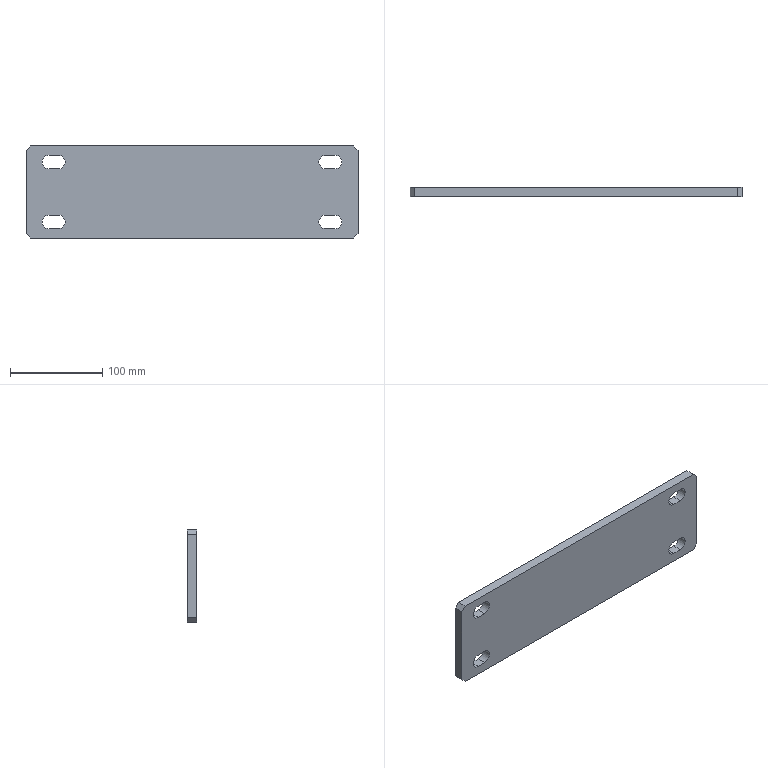Part | STEP file | Diagonal Brace连接Plate 2-2 | 1 solid | 26 faces | box 360 x 10 x 100 mm | volume 346431 mm3 | plane 18 | cylinder 8 | commonest cylinder face diameters 15 x8